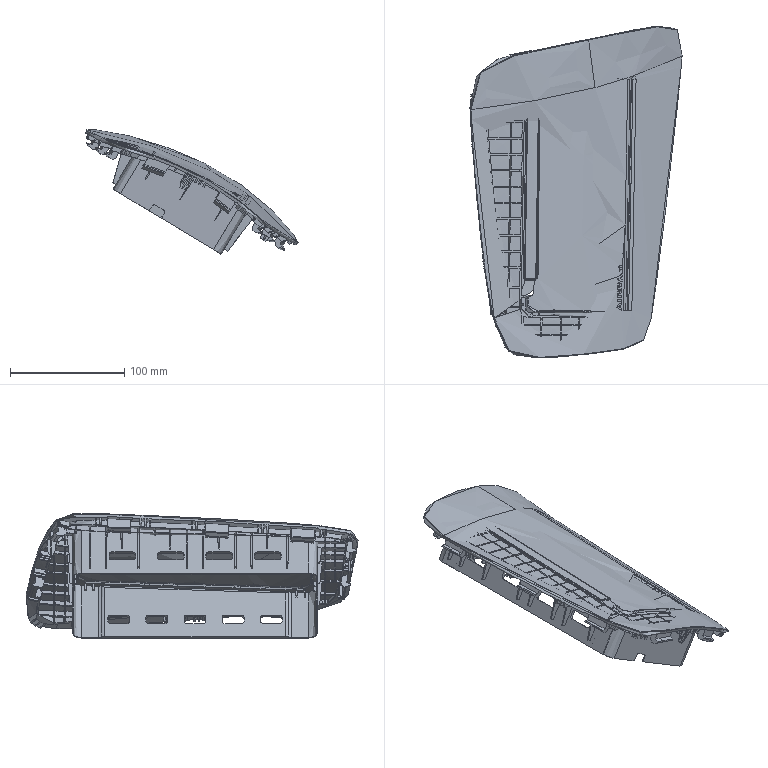Part | STEP file | 20110925@CORE-RH | 1 solid | 1916 faces | box 186.272 x 292.181 x 109.099 mm | volume 237694 mm3 | spline 1491 | plane 336 | cylinder 63 | other 12 | cone 8 | sphere 6 | commonest cylinder face diameters 5.06 x36 4.048 x10 10.12 x8 1.012 x4 6.477 x2 9.715 x2